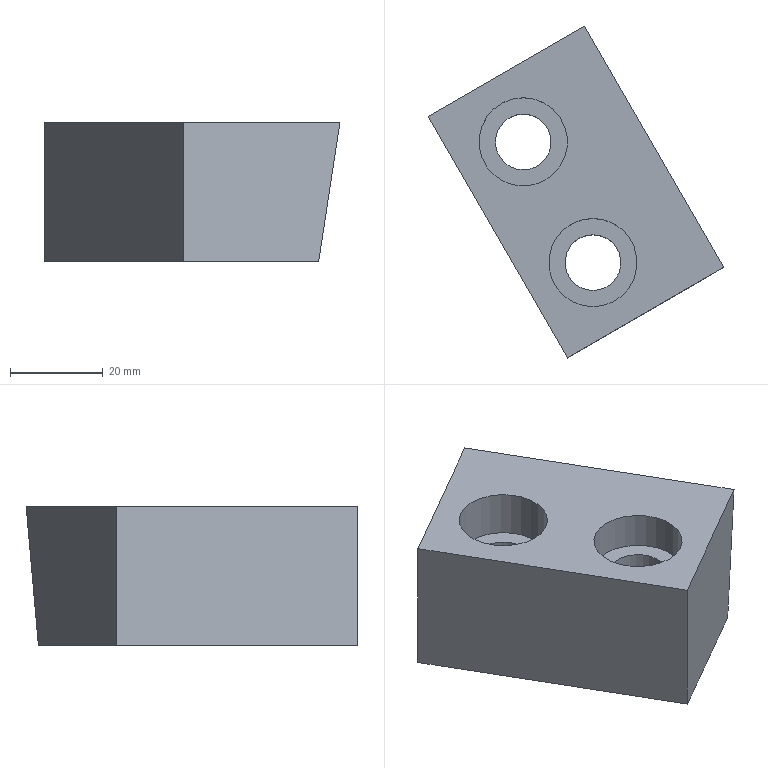Part | NX | features solid 2 | 1 solid | 12 faces | box 63.684 x 71.409 x 30 mm | volume 55424 mm3 | plane 8 | cylinder 4 | commonest cylinder face diameters 12 x2 19 x2
STEP:
#1=CARTESIAN_POINT('',(-1147.902,-59.583,-25.));
#2=VERTEX_POINT('',#1);
#3=CARTESIAN_POINT('',(-1114.217,-40.136,-25.));
#4=VERTEX_POINT('',#3);
#5=CARTESIAN_POINT('',(-1042.834,1.077,-25.));
#6=DIRECTION('',(0.866,0.5,0.));
#7=VECTOR('',#6,1000.);
#8=LINE('',#5,#7);
#9=EDGE_CURVE('',#2,#4,#8,.T.);
#10=ORIENTED_EDGE('',*,*,#9,.F.);
#11=CARTESIAN_POINT('',(-1147.902,-59.583,-55.));
#12=VERTEX_POINT('',#11);
#13=CARTESIAN_POINT('',(-1147.902,-59.583,-74.986));
#14=DIRECTION('',(0.,0.,-1.));
#15=VECTOR('',#14,1000.);
#16=LINE('',#13,#15);
#17=EDGE_CURVE('',#2,#12,#16,.T.);
#18=ORIENTED_EDGE('',*,*,#17,.T.);
#19=CARTESIAN_POINT('',(-1118.799,-42.781,-55.));
#20=VERTEX_POINT('',#19);
#21=CARTESIAN_POINT('',(-1042.834,1.077,-55.));
#22=DIRECTION('',(0.866,0.5,0.));
#23=VECTOR('',#22,1000.);
#24=LINE('',#21,#23);
#25=EDGE_CURVE('',#12,#20,#24,.T.);
#26=ORIENTED_EDGE('',*,*,#25,.T.);
#27=CARTESIAN_POINT('',(-1097.318,-30.379,85.668));
#28=DIRECTION('',(0.1504,0.08682,0.9848));
#29=VECTOR('',#28,1000.);
#30=LINE('',#27,#29);
#31=EDGE_CURVE('',#20,#4,#30,.T.);
#32=ORIENTED_EDGE('',*,*,#31,.T.);
#33=EDGE_LOOP('',(#10,#18,#26,#32));
#34=FACE_BOUND('',#33,.T.);
#35=CARTESIAN_POINT('',(-1042.834,1.077,-74.986));
#36=DIRECTION('',(0.5,-0.866,0.));
#37=DIRECTION('',(-0.07548,-0.04358,-0.9962));
#38=AXIS2_PLACEMENT_3D('',#35,#36,#37);
#39=PLANE('',#38);
#40=ADVANCED_FACE('',(#34),#39,.T.);
#41=CARTESIAN_POINT('',(-1177.902,-7.622,-25.));
#42=VERTEX_POINT('',#41);
#43=CARTESIAN_POINT('',(-1177.902,-7.622,-55.));
#44=VERTEX_POINT('',#43);
#45=CARTESIAN_POINT('',(-1177.902,-7.622,-46.968));
#46=DIRECTION('',(0.,0.,1.));
#47=VECTOR('',#46,1000.);
#48=LINE('',#45,#47);
#49=EDGE_CURVE('',#42,#44,#48,.F.);
#50=ORIENTED_EDGE('',*,*,#49,.F.);
#51=CARTESIAN_POINT('',(-1144.217,11.826,-25.));
#52=VERTEX_POINT('',#51);
#53=CARTESIAN_POINT('',(-1106.741,33.463,-25.));
#54=DIRECTION('',(-0.866,-0.5,0.));
#55=VECTOR('',#54,1000.);
#56=LINE('',#53,#55);
#57=EDGE_CURVE('',#42,#52,#56,.F.);
#58=ORIENTED_EDGE('',*,*,#57,.T.);
#59=CARTESIAN_POINT('',(-1148.799,9.181,-55.));
#60=VERTEX_POINT('',#59);
#61=CARTESIAN_POINT('',(-1149.468,8.795,-59.383));
#62=DIRECTION('',(-0.1504,-0.08682,-0.9848));
#63=VECTOR('',#62,1000.);
#64=LINE('',#61,#63);
#65=EDGE_CURVE('',#60,#52,#64,.F.);
#66=ORIENTED_EDGE('',*,*,#65,.F.);
#67=CARTESIAN_POINT('',(-1110.969,31.022,-55.));
#68=DIRECTION('',(-0.866,-0.5,0.));
#69=VECTOR('',#68,1000.);
#70=LINE('',#67,#69);
#71=EDGE_CURVE('',#44,#60,#70,.F.);
#72=ORIENTED_EDGE('',*,*,#71,.F.);
#73=EDGE_LOOP('',(#50,#58,#66,#72));
#74=FACE_BOUND('',#73,.T.);
#75=CARTESIAN_POINT('',(-1072.834,53.039,-74.986));
#76=DIRECTION('',(0.5,-0.866,0.));
#77=DIRECTION('',(-0.07548,-0.04358,-0.9962));
#78=AXIS2_PLACEMENT_3D('',#75,#76,#77);
#79=PLANE('',#78);
#80=ADVANCED_FACE('',(#74),#79,.F.);
#81=CARTESIAN_POINT('',(-1072.759,-111.945,-25.));
#82=DIRECTION('',(0.5,-0.866,0.));
#83=VECTOR('',#82,1000.);
#84=LINE('',#81,#83);
#85=EDGE_CURVE('',#52,#4,#84,.T.);
#86=ORIENTED_EDGE('',*,*,#85,.T.);
#87=ORIENTED_EDGE('',*,*,#31,.F.);
#88=CARTESIAN_POINT('',(-1077.34,-114.59,-55.));
#89=DIRECTION('',(0.5,-0.866,0.));
#90=VECTOR('',#89,1000.);
#91=LINE('',#88,#90);
#92=EDGE_CURVE('',#60,#20,#91,.T.);
#93=ORIENTED_EDGE('',*,*,#92,.F.);
#94=ORIENTED_EDGE('',*,*,#65,.T.);
#95=EDGE_LOOP('',(#86,#87,#93,#94));
#96=FACE_BOUND('',#95,.T.);
#97=CARTESIAN_POINT('',(-1055.859,-102.188,85.668));
#98=DIRECTION('',(-0.8529,-0.4924,0.1736));
#99=DIRECTION('',(0.1504,0.08682,0.9848));
#100=AXIS2_PLACEMENT_3D('',#97,#98,#99);
#101=PLANE('',#100);
#102=ADVANCED_FACE('',(#96),#101,.F.);
#103=CARTESIAN_POINT('',(-1142.411,-33.093,-55.));
#104=VERTEX_POINT('',#103);
#105=CARTESIAN_POINT('',(-1142.411,-39.093,-55.));
#106=DIRECTION('',(0.,0.,-1.));
#107=DIRECTION('',(0.,1.,0.));
#108=AXIS2_PLACEMENT_3D('',#105,#106,#107);
#109=CIRCLE('',#108,6.);
#110=EDGE_CURVE('',#104,#104,#109,.F.);
#111=ORIENTED_EDGE('',*,*,#110,.T.);
#112=EDGE_LOOP('',(#111));
#113=FACE_BOUND('',#112,.T.);
#114=CARTESIAN_POINT('',(-1157.411,-7.112,-55.));
#115=VERTEX_POINT('',#114);
#116=CARTESIAN_POINT('',(-1157.411,-13.112,-55.));
#117=DIRECTION('',(0.,0.,-1.));
#118=DIRECTION('',(0.,1.,0.));
#119=AXIS2_PLACEMENT_3D('',#116,#117,#118);
#120=CIRCLE('',#119,6.);
#121=EDGE_CURVE('',#115,#115,#120,.F.);
#122=ORIENTED_EDGE('',*,*,#121,.T.);
#123=EDGE_LOOP('',(#122));
#124=FACE_BOUND('',#123,.T.);
#125=ORIENTED_EDGE('',*,*,#71,.T.);
#126=ORIENTED_EDGE('',*,*,#92,.T.);
#127=ORIENTED_EDGE('',*,*,#25,.F.);
#128=CARTESIAN_POINT('',(-1177.902,-7.622,-55.));
#129=DIRECTION('',(0.5,-0.866,0.));
#130=VECTOR('',#129,1000.);
#131=LINE('',#128,#130);
#132=EDGE_CURVE('',#44,#12,#131,.T.);
#133=ORIENTED_EDGE('',*,*,#132,.F.);
#134=EDGE_LOOP('',(#125,#126,#127,#133));
#135=FACE_BOUND('',#134,.T.);
#136=CARTESIAN_POINT('',(-1098.469,9.371,-55.));
#137=DIRECTION('',(0.,0.,-1.));
#138=DIRECTION('',(0.,1.,0.));
#139=AXIS2_PLACEMENT_3D('',#136,#137,#138);
#140=PLANE('',#139);
#141=ADVANCED_FACE('',(#113,#124,#135),#140,.T.);
#142=CARTESIAN_POINT('',(-1142.411,-29.593,-25.));
#143=VERTEX_POINT('',#142);
#144=CARTESIAN_POINT('',(-1142.411,-39.093,-25.));
#145=DIRECTION('',(0.,0.,-1.));
#146=DIRECTION('',(0.,1.,0.));
#147=AXIS2_PLACEMENT_3D('',#144,#145,#146);
#148=CIRCLE('',#147,9.5);
#149=EDGE_CURVE('',#143,#143,#148,.F.);
#150=ORIENTED_EDGE('',*,*,#149,.F.);
#151=EDGE_LOOP('',(#150));
#152=FACE_BOUND('',#151,.T.);
#153=CARTESIAN_POINT('',(-1157.411,-3.612,-25.));
#154=VERTEX_POINT('',#153);
#155=CARTESIAN_POINT('',(-1157.411,-13.112,-25.));
#156=DIRECTION('',(0.,0.,-1.));
#157=DIRECTION('',(0.,1.,0.));
#158=AXIS2_PLACEMENT_3D('',#155,#156,#157);
#159=CIRCLE('',#158,9.5);
#160=EDGE_CURVE('',#154,#154,#159,.F.);
#161=ORIENTED_EDGE('',*,*,#160,.F.);
#162=EDGE_LOOP('',(#161));
#163=FACE_BOUND('',#162,.T.);
#164=CARTESIAN_POINT('',(-1165.402,-29.272,-25.));
#165=DIRECTION('',(-0.5,0.866,0.));
#166=VECTOR('',#165,1000.);
#167=LINE('',#164,#166);
#168=EDGE_CURVE('',#2,#42,#167,.T.);
#169=ORIENTED_EDGE('',*,*,#168,.F.);
#170=ORIENTED_EDGE('',*,*,#9,.T.);
#171=ORIENTED_EDGE('',*,*,#85,.F.);
#172=ORIENTED_EDGE('',*,*,#57,.F.);
#173=EDGE_LOOP('',(#169,#170,#171,#172));
#174=FACE_BOUND('',#173,.T.);
#175=CARTESIAN_POINT('',(-1094.241,11.812,-25.));
#176=DIRECTION('',(0.,0.,-1.));
#177=DIRECTION('',(0.,1.,0.));
#178=AXIS2_PLACEMENT_3D('',#175,#176,#177);
#179=PLANE('',#178);
#180=ADVANCED_FACE('',(#152,#163,#174),#179,.F.);
#181=ORIENTED_EDGE('',*,*,#168,.T.);
#182=ORIENTED_EDGE('',*,*,#49,.T.);
#183=ORIENTED_EDGE('',*,*,#132,.T.);
#184=ORIENTED_EDGE('',*,*,#17,.F.);
#185=EDGE_LOOP('',(#181,#182,#183,#184));
#186=FACE_BOUND('',#185,.T.);
#187=CARTESIAN_POINT('',(-1177.902,-7.622,-46.968));
#188=DIRECTION('',(-0.866,-0.5,0.));
#189=DIRECTION('',(0.5,-0.866,0.));
#190=AXIS2_PLACEMENT_3D('',#187,#188,#189);
#191=PLANE('',#190);
#192=ADVANCED_FACE('',(#186),#191,.T.);
#193=CARTESIAN_POINT('',(-1157.411,-7.112,-35.));
#194=VERTEX_POINT('',#193);
#195=CARTESIAN_POINT('',(-1157.411,-13.112,-35.));
#196=DIRECTION('',(0.,0.,-1.));
#197=DIRECTION('',(0.,1.,0.));
#198=AXIS2_PLACEMENT_3D('',#195,#196,#197);
#199=CIRCLE('',#198,6.);
#200=EDGE_CURVE('',#194,#194,#199,.F.);
#201=ORIENTED_EDGE('',*,*,#200,.T.);
#202=EDGE_LOOP('',(#201));
#203=FACE_BOUND('',#202,.T.);
#204=ORIENTED_EDGE('',*,*,#121,.F.);
#205=EDGE_LOOP('',(#204));
#206=FACE_BOUND('',#205,.T.);
#207=CARTESIAN_POINT('',(-1157.411,-13.112,-72.844));
#208=DIRECTION('',(0.,0.,1.));
#209=DIRECTION('',(0.,-1.,0.));
#210=AXIS2_PLACEMENT_3D('',#207,#208,#209);
#211=CYLINDRICAL_SURFACE('',#210,6.);
#212=ADVANCED_FACE('',(#203,#206),#211,.F.);
#213=ORIENTED_EDGE('',*,*,#200,.F.);
#214=EDGE_LOOP('',(#213));
#215=FACE_BOUND('',#214,.T.);
#216=CARTESIAN_POINT('',(-1157.411,-3.612,-35.));
#217=VERTEX_POINT('',#216);
#218=CARTESIAN_POINT('',(-1157.411,-13.112,-35.));
#219=DIRECTION('',(0.,0.,-1.));
#220=DIRECTION('',(0.,1.,0.));
#221=AXIS2_PLACEMENT_3D('',#218,#219,#220);
#222=CIRCLE('',#221,9.5);
#223=EDGE_CURVE('',#217,#217,#222,.F.);
#224=ORIENTED_EDGE('',*,*,#223,.T.);
#225=EDGE_LOOP('',(#224));
#226=FACE_BOUND('',#225,.T.);
#227=CARTESIAN_POINT('',(-1160.,-12.,-35.));
#228=DIRECTION('',(0.,0.,-1.));
#229=DIRECTION('',(0.,1.,0.));
#230=AXIS2_PLACEMENT_3D('',#227,#228,#229);
#231=PLANE('',#230);
#232=ADVANCED_FACE('',(#215,#226),#231,.F.);
#233=ORIENTED_EDGE('',*,*,#160,.T.);
#234=EDGE_LOOP('',(#233));
#235=FACE_BOUND('',#234,.T.);
#236=ORIENTED_EDGE('',*,*,#223,.F.);
#237=EDGE_LOOP('',(#236));
#238=FACE_BOUND('',#237,.T.);
#239=CARTESIAN_POINT('',(-1157.411,-13.112,-32.844));
#240=DIRECTION('',(0.,0.,1.));
#241=DIRECTION('',(0.,-1.,0.));
#242=AXIS2_PLACEMENT_3D('',#239,#240,#241);
#243=CYLINDRICAL_SURFACE('',#242,9.5);
#244=ADVANCED_FACE('',(#235,#238),#243,.F.);
#245=CARTESIAN_POINT('',(-1142.411,-33.093,-32.844));
#246=VERTEX_POINT('',#245);
#247=CARTESIAN_POINT('',(-1142.411,-39.093,-32.844));
#248=DIRECTION('',(0.,0.,-1.));
#249=DIRECTION('',(0.,1.,0.));
#250=AXIS2_PLACEMENT_3D('',#247,#248,#249);
#251=CIRCLE('',#250,6.);
#252=EDGE_CURVE('',#246,#246,#251,.F.);
#253=ORIENTED_EDGE('',*,*,#252,.T.);
#254=EDGE_LOOP('',(#253));
#255=FACE_BOUND('',#254,.T.);
#256=ORIENTED_EDGE('',*,*,#110,.F.);
#257=EDGE_LOOP('',(#256));
#258=FACE_BOUND('',#257,.T.);
#259=CARTESIAN_POINT('',(-1142.411,-39.093,-72.844));
#260=DIRECTION('',(0.,0.,1.));
#261=DIRECTION('',(0.,-1.,0.));
#262=AXIS2_PLACEMENT_3D('',#259,#260,#261);
#263=CYLINDRICAL_SURFACE('',#262,6.);
#264=ADVANCED_FACE('',(#255,#258),#263,.F.);
#265=ORIENTED_EDGE('',*,*,#252,.F.);
#266=EDGE_LOOP('',(#265));
#267=FACE_BOUND('',#266,.T.);
#268=CARTESIAN_POINT('',(-1142.411,-48.593,-32.844));
#269=VERTEX_POINT('',#268);
#270=CARTESIAN_POINT('',(-1142.411,-39.093,-32.844));
#271=DIRECTION('',(0.,0.,1.));
#272=DIRECTION('',(0.,-1.,0.));
#273=AXIS2_PLACEMENT_3D('',#270,#271,#272);
#274=CIRCLE('',#273,9.5);
#275=EDGE_CURVE('',#269,#269,#274,.T.);
#276=ORIENTED_EDGE('',*,*,#275,.T.);
#277=EDGE_LOOP('',(#276));
#278=FACE_BOUND('',#277,.T.);
#279=CARTESIAN_POINT('',(-1143.,-40.,-32.844));
#280=DIRECTION('',(0.,0.,-1.));
#281=DIRECTION('',(0.,1.,0.));
#282=AXIS2_PLACEMENT_3D('',#279,#280,#281);
#283=PLANE('',#282);
#284=ADVANCED_FACE('',(#267,#278),#283,.F.);
#285=ORIENTED_EDGE('',*,*,#149,.T.);
#286=EDGE_LOOP('',(#285));
#287=FACE_BOUND('',#286,.T.);
#288=ORIENTED_EDGE('',*,*,#275,.F.);
#289=EDGE_LOOP('',(#288));
#290=FACE_BOUND('',#289,.T.);
#291=CARTESIAN_POINT('',(-1142.411,-39.093,-32.844));
#292=DIRECTION('',(0.,0.,1.));
#293=DIRECTION('',(0.,-1.,0.));
#294=AXIS2_PLACEMENT_3D('',#291,#292,#293);
#295=CYLINDRICAL_SURFACE('',#294,9.5);
#296=ADVANCED_FACE('',(#287,#290),#295,.F.);
#297=CLOSED_SHELL('',(#40,#80,#102,#141,#180,#192,#212,#232,#244,#264,#284,#296));
#298=MANIFOLD_SOLID_BREP('',#297);
#299=(LENGTH_UNIT()NAMED_UNIT(*)SI_UNIT(.MILLI.,.METRE.));
#300=UNCERTAINTY_MEASURE_WITH_UNIT(LENGTH_MEASURE(0.00001),#299,'','');
#301=(NAMED_UNIT(*)PLANE_ANGLE_UNIT()SI_UNIT($,.RADIAN.));
#302=(NAMED_UNIT(*)SI_UNIT($,.STERADIAN.)SOLID_ANGLE_UNIT());
#303=(GEOMETRIC_REPRESENTATION_CONTEXT(3)GLOBAL_UNCERTAINTY_ASSIGNED_CONTEXT((#300))GLOBAL_UNIT_ASSIGNED_CONTEXT((#299,#301,#302))REPRESENTATION_CONTEXT('',''));
#304=ADVANCED_BREP_SHAPE_REPRESENTATION('',(#298),#303);